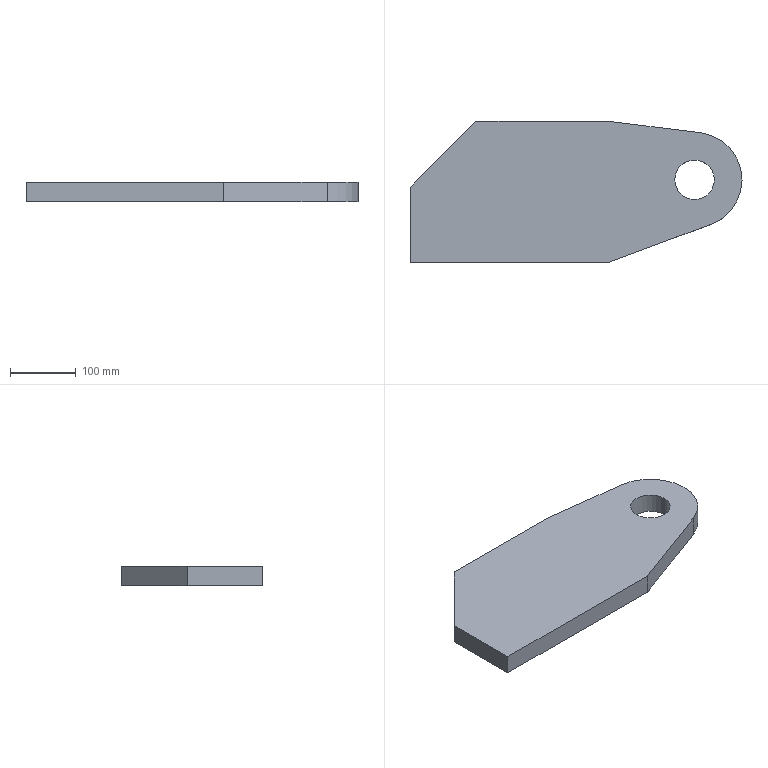Part | SolidWorks | features Extrusion 1 | 1 solid | 11 faces | box 504 x 215 x 30 mm | volume 2667245 mm3 | plane 8 | cylinder 3 | commonest cylinder face diameters 60 x2 144 x1
STEP:
#1=CARTESIAN_POINT('',(402.,126.,30.));
#2=VERTEX_POINT('',#1);
#3=CARTESIAN_POINT('',(462.,126.,30.));
#4=VERTEX_POINT('',#3);
#5=CARTESIAN_POINT('',(432.,126.,30.));
#6=DIRECTION('',(0.,0.,1.));
#7=DIRECTION('',(1.,0.,0.));
#8=AXIS2_PLACEMENT_3D('',#5,#6,#7);
#9=CIRCLE('',#8,30.);
#10=EDGE_CURVE('',#2,#4,#9,.T.);
#11=ORIENTED_EDGE('',*,*,#10,.T.);
#12=CARTESIAN_POINT('',(462.,126.,0.));
#13=VERTEX_POINT('',#12);
#14=CARTESIAN_POINT('',(462.,126.,30.));
#15=DIRECTION('',(0.,0.,-1.));
#16=VECTOR('',#15,1000.);
#17=LINE('',#14,#16);
#18=EDGE_CURVE('',#4,#13,#17,.T.);
#19=ORIENTED_EDGE('',*,*,#18,.T.);
#20=CARTESIAN_POINT('',(402.,126.,0.));
#21=VERTEX_POINT('',#20);
#22=CARTESIAN_POINT('',(432.,126.,0.));
#23=DIRECTION('',(0.,0.,1.));
#24=DIRECTION('',(1.,0.,0.));
#25=AXIS2_PLACEMENT_3D('',#22,#23,#24);
#26=CIRCLE('',#25,30.);
#27=EDGE_CURVE('',#21,#13,#26,.T.);
#28=ORIENTED_EDGE('',*,*,#27,.F.);
#29=CARTESIAN_POINT('',(402.,126.,30.));
#30=DIRECTION('',(0.,0.,-1.));
#31=VECTOR('',#30,1000.);
#32=LINE('',#29,#31);
#33=EDGE_CURVE('',#2,#21,#32,.T.);
#34=ORIENTED_EDGE('',*,*,#33,.F.);
#35=EDGE_LOOP('',(#11,#19,#28,#34));
#36=FACE_OUTER_BOUND('',#35,.T.);
#37=CARTESIAN_POINT('',(432.,126.,30.));
#38=DIRECTION('',(0.,0.,-1.));
#39=DIRECTION('',(-1.,0.,0.));
#40=AXIS2_PLACEMENT_3D('',#37,#38,#39);
#41=CYLINDRICAL_SURFACE('',#40,30.);
#42=ADVANCED_FACE('',(#36),#41,.F.);
#43=CARTESIAN_POINT('',(0.,115.,30.));
#44=VERTEX_POINT('',#43);
#45=CARTESIAN_POINT('',(0.,0.,30.));
#46=VERTEX_POINT('',#45);
#47=CARTESIAN_POINT('',(0.,115.,30.));
#48=DIRECTION('',(0.,-1.,0.));
#49=VECTOR('',#48,1000.);
#50=LINE('',#47,#49);
#51=EDGE_CURVE('',#44,#46,#50,.T.);
#52=ORIENTED_EDGE('',*,*,#51,.T.);
#53=CARTESIAN_POINT('',(300.,0.,30.));
#54=VERTEX_POINT('',#53);
#55=CARTESIAN_POINT('',(0.,0.,30.));
#56=DIRECTION('',(1.,0.,0.));
#57=VECTOR('',#56,1000.);
#58=LINE('',#55,#57);
#59=EDGE_CURVE('',#46,#54,#58,.T.);
#60=ORIENTED_EDGE('',*,*,#59,.T.);
#61=CARTESIAN_POINT('',(457.132,58.529,30.));
#62=VERTEX_POINT('',#61);
#63=CARTESIAN_POINT('',(300.,0.,30.));
#64=DIRECTION('',(0.9371,0.3491,0.));
#65=VECTOR('',#64,1000.);
#66=LINE('',#63,#65);
#67=EDGE_CURVE('',#54,#62,#66,.T.);
#68=ORIENTED_EDGE('',*,*,#67,.T.);
#69=CARTESIAN_POINT('',(440.9,197.448,30.));
#70=VERTEX_POINT('',#69);
#71=CARTESIAN_POINT('',(432.,126.,30.));
#72=DIRECTION('',(0.,0.,1.));
#73=DIRECTION('',(1.,0.,0.));
#74=AXIS2_PLACEMENT_3D('',#71,#72,#73);
#75=CIRCLE('',#74,72.);
#76=EDGE_CURVE('',#62,#70,#75,.T.);
#77=ORIENTED_EDGE('',*,*,#76,.T.);
#78=CARTESIAN_POINT('',(300.,215.,30.));
#79=VERTEX_POINT('',#78);
#80=CARTESIAN_POINT('',(440.9,197.448,30.));
#81=DIRECTION('',(-0.9923,0.1236,0.));
#82=VECTOR('',#81,1000.);
#83=LINE('',#80,#82);
#84=EDGE_CURVE('',#70,#79,#83,.T.);
#85=ORIENTED_EDGE('',*,*,#84,.T.);
#86=CARTESIAN_POINT('',(100.,215.,30.));
#87=VERTEX_POINT('',#86);
#88=CARTESIAN_POINT('',(300.,215.,30.));
#89=DIRECTION('',(-1.,0.,0.));
#90=VECTOR('',#89,1000.);
#91=LINE('',#88,#90);
#92=EDGE_CURVE('',#79,#87,#91,.T.);
#93=ORIENTED_EDGE('',*,*,#92,.T.);
#94=CARTESIAN_POINT('',(100.,215.,30.));
#95=DIRECTION('',(-0.7071,-0.7071,0.));
#96=VECTOR('',#95,1000.);
#97=LINE('',#94,#96);
#98=EDGE_CURVE('',#87,#44,#97,.T.);
#99=ORIENTED_EDGE('',*,*,#98,.T.);
#100=EDGE_LOOP('',(#52,#60,#68,#77,#85,#93,#99));
#101=FACE_OUTER_BOUND('',#100,.T.);
#102=ORIENTED_EDGE('',*,*,#10,.F.);
#103=CARTESIAN_POINT('',(432.,126.,30.));
#104=DIRECTION('',(0.,0.,1.));
#105=DIRECTION('',(1.,0.,0.));
#106=AXIS2_PLACEMENT_3D('',#103,#104,#105);
#107=CIRCLE('',#106,30.);
#108=EDGE_CURVE('',#4,#2,#107,.T.);
#109=ORIENTED_EDGE('',*,*,#108,.F.);
#110=EDGE_LOOP('',(#102,#109));
#111=FACE_BOUND('',#110,.T.);
#112=CARTESIAN_POINT('',(432.,126.,30.));
#113=DIRECTION('',(0.,0.,1.));
#114=DIRECTION('',(1.,0.,0.));
#115=AXIS2_PLACEMENT_3D('',#112,#113,#114);
#116=PLANE('',#115);
#117=ADVANCED_FACE('',(#101,#111),#116,.T.);
#118=CARTESIAN_POINT('',(0.,115.,0.));
#119=VERTEX_POINT('',#118);
#120=CARTESIAN_POINT('',(0.,0.,0.));
#121=VERTEX_POINT('',#120);
#122=CARTESIAN_POINT('',(0.,115.,0.));
#123=DIRECTION('',(0.,-1.,0.));
#124=VECTOR('',#123,1000.);
#125=LINE('',#122,#124);
#126=EDGE_CURVE('',#119,#121,#125,.T.);
#127=ORIENTED_EDGE('',*,*,#126,.F.);
#128=CARTESIAN_POINT('',(100.,215.,0.));
#129=VERTEX_POINT('',#128);
#130=CARTESIAN_POINT('',(100.,215.,0.));
#131=DIRECTION('',(-0.7071,-0.7071,0.));
#132=VECTOR('',#131,1000.);
#133=LINE('',#130,#132);
#134=EDGE_CURVE('',#129,#119,#133,.T.);
#135=ORIENTED_EDGE('',*,*,#134,.F.);
#136=CARTESIAN_POINT('',(300.,215.,0.));
#137=VERTEX_POINT('',#136);
#138=CARTESIAN_POINT('',(300.,215.,0.));
#139=DIRECTION('',(-1.,0.,0.));
#140=VECTOR('',#139,1000.);
#141=LINE('',#138,#140);
#142=EDGE_CURVE('',#137,#129,#141,.T.);
#143=ORIENTED_EDGE('',*,*,#142,.F.);
#144=CARTESIAN_POINT('',(440.9,197.448,0.));
#145=VERTEX_POINT('',#144);
#146=CARTESIAN_POINT('',(440.9,197.448,0.));
#147=DIRECTION('',(-0.9923,0.1236,0.));
#148=VECTOR('',#147,1000.);
#149=LINE('',#146,#148);
#150=EDGE_CURVE('',#145,#137,#149,.T.);
#151=ORIENTED_EDGE('',*,*,#150,.F.);
#152=CARTESIAN_POINT('',(457.132,58.529,0.));
#153=VERTEX_POINT('',#152);
#154=CARTESIAN_POINT('',(432.,126.,0.));
#155=DIRECTION('',(0.,0.,1.));
#156=DIRECTION('',(1.,0.,0.));
#157=AXIS2_PLACEMENT_3D('',#154,#155,#156);
#158=CIRCLE('',#157,72.);
#159=EDGE_CURVE('',#153,#145,#158,.T.);
#160=ORIENTED_EDGE('',*,*,#159,.F.);
#161=CARTESIAN_POINT('',(300.,0.,0.));
#162=VERTEX_POINT('',#161);
#163=CARTESIAN_POINT('',(300.,0.,0.));
#164=DIRECTION('',(0.9371,0.3491,0.));
#165=VECTOR('',#164,1000.);
#166=LINE('',#163,#165);
#167=EDGE_CURVE('',#162,#153,#166,.T.);
#168=ORIENTED_EDGE('',*,*,#167,.F.);
#169=CARTESIAN_POINT('',(0.,0.,0.));
#170=DIRECTION('',(1.,0.,0.));
#171=VECTOR('',#170,1000.);
#172=LINE('',#169,#171);
#173=EDGE_CURVE('',#121,#162,#172,.T.);
#174=ORIENTED_EDGE('',*,*,#173,.F.);
#175=EDGE_LOOP('',(#127,#135,#143,#151,#160,#168,#174));
#176=FACE_OUTER_BOUND('',#175,.T.);
#177=ORIENTED_EDGE('',*,*,#27,.T.);
#178=CARTESIAN_POINT('',(432.,126.,0.));
#179=DIRECTION('',(0.,0.,1.));
#180=DIRECTION('',(1.,0.,0.));
#181=AXIS2_PLACEMENT_3D('',#178,#179,#180);
#182=CIRCLE('',#181,30.);
#183=EDGE_CURVE('',#13,#21,#182,.T.);
#184=ORIENTED_EDGE('',*,*,#183,.T.);
#185=EDGE_LOOP('',(#177,#184));
#186=FACE_BOUND('',#185,.T.);
#187=CARTESIAN_POINT('',(432.,126.,0.));
#188=DIRECTION('',(0.,0.,1.));
#189=DIRECTION('',(1.,0.,0.));
#190=AXIS2_PLACEMENT_3D('',#187,#188,#189);
#191=PLANE('',#190);
#192=ADVANCED_FACE('',(#176,#186),#191,.F.);
#193=ORIENTED_EDGE('',*,*,#126,.T.);
#194=CARTESIAN_POINT('',(0.,0.,30.));
#195=DIRECTION('',(0.,0.,-1.));
#196=VECTOR('',#195,1000.);
#197=LINE('',#194,#196);
#198=EDGE_CURVE('',#46,#121,#197,.T.);
#199=ORIENTED_EDGE('',*,*,#198,.F.);
#200=ORIENTED_EDGE('',*,*,#51,.F.);
#201=CARTESIAN_POINT('',(0.,115.,30.));
#202=DIRECTION('',(0.,0.,-1.));
#203=VECTOR('',#202,1000.);
#204=LINE('',#201,#203);
#205=EDGE_CURVE('',#44,#119,#204,.T.);
#206=ORIENTED_EDGE('',*,*,#205,.T.);
#207=EDGE_LOOP('',(#193,#199,#200,#206));
#208=FACE_OUTER_BOUND('',#207,.T.);
#209=CARTESIAN_POINT('',(0.,115.,30.));
#210=DIRECTION('',(1.,0.,0.));
#211=DIRECTION('',(0.,1.,0.));
#212=AXIS2_PLACEMENT_3D('',#209,#210,#211);
#213=PLANE('',#212);
#214=ADVANCED_FACE('',(#208),#213,.F.);
#215=ORIENTED_EDGE('',*,*,#173,.T.);
#216=CARTESIAN_POINT('',(300.,0.,30.));
#217=DIRECTION('',(0.,0.,-1.));
#218=VECTOR('',#217,1000.);
#219=LINE('',#216,#218);
#220=EDGE_CURVE('',#54,#162,#219,.T.);
#221=ORIENTED_EDGE('',*,*,#220,.F.);
#222=ORIENTED_EDGE('',*,*,#59,.F.);
#223=ORIENTED_EDGE('',*,*,#198,.T.);
#224=EDGE_LOOP('',(#215,#221,#222,#223));
#225=FACE_OUTER_BOUND('',#224,.T.);
#226=CARTESIAN_POINT('',(0.,0.,30.));
#227=DIRECTION('',(0.,1.,0.));
#228=DIRECTION('',(0.,0.,1.));
#229=AXIS2_PLACEMENT_3D('',#226,#227,#228);
#230=PLANE('',#229);
#231=ADVANCED_FACE('',(#225),#230,.F.);
#232=ORIENTED_EDGE('',*,*,#167,.T.);
#233=CARTESIAN_POINT('',(457.132,58.529,30.));
#234=DIRECTION('',(0.,0.,-1.));
#235=VECTOR('',#234,1000.);
#236=LINE('',#233,#235);
#237=EDGE_CURVE('',#62,#153,#236,.T.);
#238=ORIENTED_EDGE('',*,*,#237,.F.);
#239=ORIENTED_EDGE('',*,*,#67,.F.);
#240=ORIENTED_EDGE('',*,*,#220,.T.);
#241=EDGE_LOOP('',(#232,#238,#239,#240));
#242=FACE_OUTER_BOUND('',#241,.T.);
#243=CARTESIAN_POINT('',(300.,0.,30.));
#244=DIRECTION('',(-0.3491,0.9371,0.));
#245=DIRECTION('',(-0.9371,-0.3491,0.));
#246=AXIS2_PLACEMENT_3D('',#243,#244,#245);
#247=PLANE('',#246);
#248=ADVANCED_FACE('',(#242),#247,.F.);
#249=ORIENTED_EDGE('',*,*,#159,.T.);
#250=CARTESIAN_POINT('',(440.9,197.448,30.));
#251=DIRECTION('',(0.,0.,-1.));
#252=VECTOR('',#251,1000.);
#253=LINE('',#250,#252);
#254=EDGE_CURVE('',#70,#145,#253,.T.);
#255=ORIENTED_EDGE('',*,*,#254,.F.);
#256=ORIENTED_EDGE('',*,*,#76,.F.);
#257=ORIENTED_EDGE('',*,*,#237,.T.);
#258=EDGE_LOOP('',(#249,#255,#256,#257));
#259=FACE_OUTER_BOUND('',#258,.T.);
#260=CARTESIAN_POINT('',(432.,126.,30.));
#261=DIRECTION('',(0.,0.,-1.));
#262=DIRECTION('',(-1.,0.,0.));
#263=AXIS2_PLACEMENT_3D('',#260,#261,#262);
#264=CYLINDRICAL_SURFACE('',#263,72.);
#265=ADVANCED_FACE('',(#259),#264,.T.);
#266=ORIENTED_EDGE('',*,*,#150,.T.);
#267=CARTESIAN_POINT('',(300.,215.,30.));
#268=DIRECTION('',(0.,0.,-1.));
#269=VECTOR('',#268,1000.);
#270=LINE('',#267,#269);
#271=EDGE_CURVE('',#79,#137,#270,.T.);
#272=ORIENTED_EDGE('',*,*,#271,.F.);
#273=ORIENTED_EDGE('',*,*,#84,.F.);
#274=ORIENTED_EDGE('',*,*,#254,.T.);
#275=EDGE_LOOP('',(#266,#272,#273,#274));
#276=FACE_OUTER_BOUND('',#275,.T.);
#277=CARTESIAN_POINT('',(440.9,197.448,30.));
#278=DIRECTION('',(-0.1236,-0.9923,0.));
#279=DIRECTION('',(0.9923,-0.1236,0.));
#280=AXIS2_PLACEMENT_3D('',#277,#278,#279);
#281=PLANE('',#280);
#282=ADVANCED_FACE('',(#276),#281,.F.);
#283=ORIENTED_EDGE('',*,*,#142,.T.);
#284=CARTESIAN_POINT('',(100.,215.,30.));
#285=DIRECTION('',(0.,0.,-1.));
#286=VECTOR('',#285,1000.);
#287=LINE('',#284,#286);
#288=EDGE_CURVE('',#87,#129,#287,.T.);
#289=ORIENTED_EDGE('',*,*,#288,.F.);
#290=ORIENTED_EDGE('',*,*,#92,.F.);
#291=ORIENTED_EDGE('',*,*,#271,.T.);
#292=EDGE_LOOP('',(#283,#289,#290,#291));
#293=FACE_OUTER_BOUND('',#292,.T.);
#294=CARTESIAN_POINT('',(300.,215.,30.));
#295=DIRECTION('',(0.,-1.,0.));
#296=DIRECTION('',(1.,0.,0.));
#297=AXIS2_PLACEMENT_3D('',#294,#295,#296);
#298=PLANE('',#297);
#299=ADVANCED_FACE('',(#293),#298,.F.);
#300=ORIENTED_EDGE('',*,*,#134,.T.);
#301=ORIENTED_EDGE('',*,*,#205,.F.);
#302=ORIENTED_EDGE('',*,*,#98,.F.);
#303=ORIENTED_EDGE('',*,*,#288,.T.);
#304=EDGE_LOOP('',(#300,#301,#302,#303));
#305=FACE_OUTER_BOUND('',#304,.T.);
#306=CARTESIAN_POINT('',(100.,215.,30.));
#307=DIRECTION('',(0.7071,-0.7071,0.));
#308=DIRECTION('',(0.7071,0.7071,0.));
#309=AXIS2_PLACEMENT_3D('',#306,#307,#308);
#310=PLANE('',#309);
#311=ADVANCED_FACE('',(#305),#310,.F.);
#312=ORIENTED_EDGE('',*,*,#18,.F.);
#313=ORIENTED_EDGE('',*,*,#108,.T.);
#314=ORIENTED_EDGE('',*,*,#33,.T.);
#315=ORIENTED_EDGE('',*,*,#183,.F.);
#316=EDGE_LOOP('',(#312,#313,#314,#315));
#317=FACE_OUTER_BOUND('',#316,.T.);
#318=CARTESIAN_POINT('',(432.,126.,30.));
#319=DIRECTION('',(0.,0.,-1.));
#320=DIRECTION('',(-1.,0.,0.));
#321=AXIS2_PLACEMENT_3D('',#318,#319,#320);
#322=CYLINDRICAL_SURFACE('',#321,30.);
#323=ADVANCED_FACE('',(#317),#322,.F.);
#324=CLOSED_SHELL('',(#42,#117,#192,#214,#231,#248,#265,#282,#299,#311,#323));
#325=MANIFOLD_SOLID_BREP('',#324);
#326=CARTESIAN_POINT('',(0.,0.,0.));
#327=DIRECTION('',(0.,0.,1.));
#328=DIRECTION('',(1.,0.,0.));
#329=AXIS2_PLACEMENT_3D('',#326,#327,#328);
#330=(LENGTH_UNIT()NAMED_UNIT(*)SI_UNIT(.MILLI.,.METRE.));
#331=UNCERTAINTY_MEASURE_WITH_UNIT(LENGTH_MEASURE(0.00001),#330,'','');
#332=(NAMED_UNIT(*)PLANE_ANGLE_UNIT()SI_UNIT($,.RADIAN.));
#333=(NAMED_UNIT(*)SI_UNIT($,.STERADIAN.)SOLID_ANGLE_UNIT());
#334=(GEOMETRIC_REPRESENTATION_CONTEXT(3)GLOBAL_UNCERTAINTY_ASSIGNED_CONTEXT((#331))GLOBAL_UNIT_ASSIGNED_CONTEXT((#330,#332,#333))REPRESENTATION_CONTEXT('',''));
#335=ADVANCED_BREP_SHAPE_REPRESENTATION('',(#325,#329),#334);